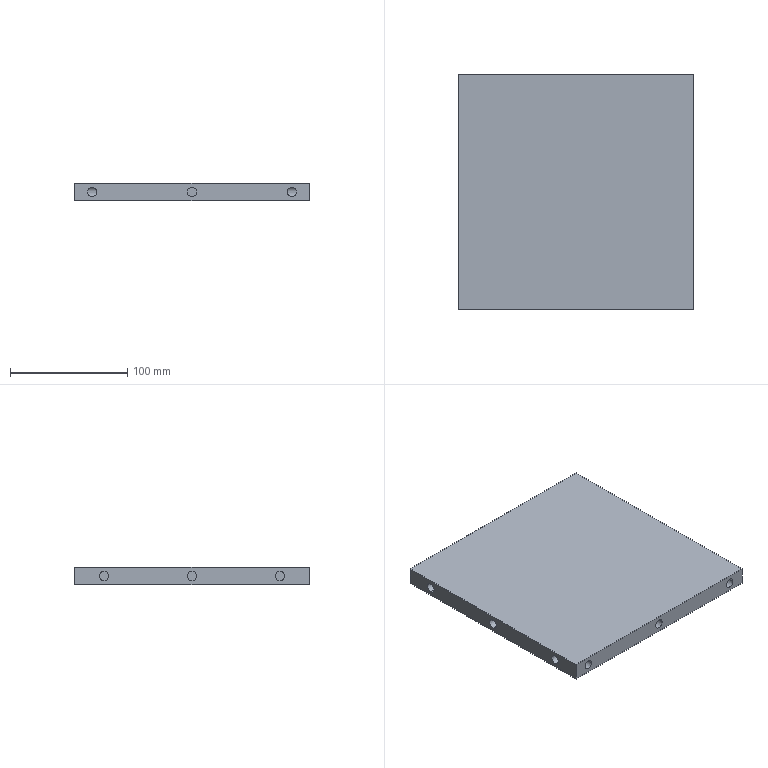Part | SolidWorks | features MirrorPattern 4, LPattern 2, Cut 1, Extrusion 1, ICE 1 | 1 solid | 42 faces | box 200 x 200 x 15 mm | volume 585603 mm3 | cylinder 28 | plane 14 | commonest cylinder face diameters 8 x28
STEP:
#1=CARTESIAN_POINT('',(-85.,-75.,3.5));
#2=VERTEX_POINT('',#1);
#3=CARTESIAN_POINT('',(-89.,-79.,7.5));
#4=VERTEX_POINT('',#3);
#5=CARTESIAN_POINT('',(-85.,-75.,3.5));
#6=CARTESIAN_POINT('',(-87.343,-77.343,3.5));
#7=CARTESIAN_POINT('',(-89.,-79.,5.157));
#8=CARTESIAN_POINT('',(-89.,-79.,7.5));
#9=(BOUNDED_CURVE()B_SPLINE_CURVE(3,(#5,#6,#7,#8),.UNSPECIFIED.,.F.,.F.)B_SPLINE_CURVE_WITH_KNOTS((4,4),(4.712,6.283),.UNSPECIFIED.)CURVE()GEOMETRIC_REPRESENTATION_ITEM()RATIONAL_B_SPLINE_CURVE((1.,0.8047,0.8047,1.))REPRESENTATION_ITEM(''));
#10=EDGE_CURVE('',#2,#4,#9,.T.);
#11=ORIENTED_EDGE('',*,*,#10,.T.);
#12=CARTESIAN_POINT('',(-89.,-100.,7.5));
#13=VERTEX_POINT('',#12);
#14=CARTESIAN_POINT('',(-89.,-75.,7.5));
#15=DIRECTION('',(0.,-1.,0.));
#16=VECTOR('',#15,1000.);
#17=LINE('',#14,#16);
#18=EDGE_CURVE('',#4,#13,#17,.T.);
#19=ORIENTED_EDGE('',*,*,#18,.T.);
#20=CARTESIAN_POINT('',(-81.,-100.,7.5));
#21=VERTEX_POINT('',#20);
#22=CARTESIAN_POINT('',(-85.,-100.,7.5));
#23=DIRECTION('',(0.,-1.,0.));
#24=DIRECTION('',(1.,0.,0.));
#25=AXIS2_PLACEMENT_3D('',#22,#23,#24);
#26=CIRCLE('',#25,4.);
#27=EDGE_CURVE('',#13,#21,#26,.T.);
#28=ORIENTED_EDGE('',*,*,#27,.T.);
#29=CARTESIAN_POINT('',(-81.,-79.,7.5));
#30=VERTEX_POINT('',#29);
#31=CARTESIAN_POINT('',(-81.,-75.,7.5));
#32=DIRECTION('',(0.,-1.,0.));
#33=VECTOR('',#32,1000.);
#34=LINE('',#31,#33);
#35=EDGE_CURVE('',#30,#21,#34,.T.);
#36=ORIENTED_EDGE('',*,*,#35,.F.);
#37=CARTESIAN_POINT('',(-81.,-79.,7.5));
#38=CARTESIAN_POINT('',(-81.,-79.,5.157));
#39=CARTESIAN_POINT('',(-82.657,-77.343,3.5));
#40=CARTESIAN_POINT('',(-85.,-75.,3.5));
#41=(BOUNDED_CURVE()B_SPLINE_CURVE(3,(#37,#38,#39,#40),.UNSPECIFIED.,.F.,.F.)B_SPLINE_CURVE_WITH_KNOTS((4,4),(3.142,4.712),.UNSPECIFIED.)CURVE()GEOMETRIC_REPRESENTATION_ITEM()RATIONAL_B_SPLINE_CURVE((1.,0.8047,0.8047,1.))REPRESENTATION_ITEM(''));
#42=EDGE_CURVE('',#30,#2,#41,.T.);
#43=ORIENTED_EDGE('',*,*,#42,.T.);
#44=EDGE_LOOP('',(#11,#19,#28,#36,#43));
#45=FACE_OUTER_BOUND('',#44,.T.);
#46=CARTESIAN_POINT('',(-85.,-75.,7.5));
#47=DIRECTION('',(0.,-1.,0.));
#48=DIRECTION('',(1.,0.,0.));
#49=AXIS2_PLACEMENT_3D('',#46,#47,#48);
#50=CYLINDRICAL_SURFACE('',#49,4.);
#51=ADVANCED_FACE('',(#45),#50,.F.);
#52=CARTESIAN_POINT('',(85.,-75.,3.5));
#53=VERTEX_POINT('',#52);
#54=CARTESIAN_POINT('',(81.,-79.,7.5));
#55=VERTEX_POINT('',#54);
#56=CARTESIAN_POINT('',(85.,-75.,3.5));
#57=CARTESIAN_POINT('',(82.657,-77.343,3.5));
#58=CARTESIAN_POINT('',(81.,-79.,5.157));
#59=CARTESIAN_POINT('',(81.,-79.,7.5));
#60=(BOUNDED_CURVE()B_SPLINE_CURVE(3,(#56,#57,#58,#59),.UNSPECIFIED.,.F.,.F.)B_SPLINE_CURVE_WITH_KNOTS((4,4),(1.571,3.142),.UNSPECIFIED.)CURVE()GEOMETRIC_REPRESENTATION_ITEM()RATIONAL_B_SPLINE_CURVE((1.,0.8047,0.8047,1.))REPRESENTATION_ITEM(''));
#61=EDGE_CURVE('',#53,#55,#60,.T.);
#62=ORIENTED_EDGE('',*,*,#61,.T.);
#63=CARTESIAN_POINT('',(81.,-100.,7.5));
#64=VERTEX_POINT('',#63);
#65=CARTESIAN_POINT('',(81.,-75.,7.5));
#66=DIRECTION('',(0.,-1.,0.));
#67=VECTOR('',#66,1000.);
#68=LINE('',#65,#67);
#69=EDGE_CURVE('',#55,#64,#68,.T.);
#70=ORIENTED_EDGE('',*,*,#69,.T.);
#71=CARTESIAN_POINT('',(89.,-100.,7.5));
#72=VERTEX_POINT('',#71);
#73=CARTESIAN_POINT('',(85.,-100.,7.5));
#74=DIRECTION('',(0.,1.,0.));
#75=DIRECTION('',(-1.,0.,0.));
#76=AXIS2_PLACEMENT_3D('',#73,#74,#75);
#77=CIRCLE('',#76,4.);
#78=EDGE_CURVE('',#72,#64,#77,.T.);
#79=ORIENTED_EDGE('',*,*,#78,.F.);
#80=CARTESIAN_POINT('',(89.,-79.,7.5));
#81=VERTEX_POINT('',#80);
#82=CARTESIAN_POINT('',(89.,-75.,7.5));
#83=DIRECTION('',(0.,-1.,0.));
#84=VECTOR('',#83,1000.);
#85=LINE('',#82,#84);
#86=EDGE_CURVE('',#81,#72,#85,.T.);
#87=ORIENTED_EDGE('',*,*,#86,.F.);
#88=CARTESIAN_POINT('',(89.,-79.,7.5));
#89=CARTESIAN_POINT('',(89.,-79.,5.157));
#90=CARTESIAN_POINT('',(87.343,-77.343,3.5));
#91=CARTESIAN_POINT('',(85.,-75.,3.5));
#92=(BOUNDED_CURVE()B_SPLINE_CURVE(3,(#88,#89,#90,#91),.UNSPECIFIED.,.F.,.F.)B_SPLINE_CURVE_WITH_KNOTS((4,4),(0.,1.571),.UNSPECIFIED.)CURVE()GEOMETRIC_REPRESENTATION_ITEM()RATIONAL_B_SPLINE_CURVE((1.,0.8047,0.8047,1.))REPRESENTATION_ITEM(''));
#93=EDGE_CURVE('',#81,#53,#92,.T.);
#94=ORIENTED_EDGE('',*,*,#93,.T.);
#95=EDGE_LOOP('',(#62,#70,#79,#87,#94));
#96=FACE_OUTER_BOUND('',#95,.T.);
#97=CARTESIAN_POINT('',(85.,-75.,7.5));
#98=DIRECTION('',(0.,-1.,0.));
#99=DIRECTION('',(1.,0.,0.));
#100=AXIS2_PLACEMENT_3D('',#97,#98,#99);
#101=CYLINDRICAL_SURFACE('',#100,4.);
#102=ADVANCED_FACE('',(#96),#101,.F.);
#103=CARTESIAN_POINT('',(4.,-75.,7.5));
#104=VERTEX_POINT('',#103);
#105=CARTESIAN_POINT('',(-4.,-75.,7.5));
#106=VERTEX_POINT('',#105);
#107=CARTESIAN_POINT('',(0.,-75.,7.5));
#108=DIRECTION('',(0.,1.,0.));
#109=DIRECTION('',(-1.,0.,0.));
#110=AXIS2_PLACEMENT_3D('',#107,#108,#109);
#111=CIRCLE('',#110,4.);
#112=EDGE_CURVE('',#104,#106,#111,.T.);
#113=ORIENTED_EDGE('',*,*,#112,.T.);
#114=CARTESIAN_POINT('',(-4.,-100.,7.5));
#115=VERTEX_POINT('',#114);
#116=CARTESIAN_POINT('',(-4.,-75.,7.5));
#117=DIRECTION('',(0.,-1.,0.));
#118=VECTOR('',#117,1000.);
#119=LINE('',#116,#118);
#120=EDGE_CURVE('',#106,#115,#119,.T.);
#121=ORIENTED_EDGE('',*,*,#120,.T.);
#122=CARTESIAN_POINT('',(4.,-100.,7.5));
#123=VERTEX_POINT('',#122);
#124=CARTESIAN_POINT('',(0.,-100.,7.5));
#125=DIRECTION('',(0.,1.,0.));
#126=DIRECTION('',(-1.,0.,0.));
#127=AXIS2_PLACEMENT_3D('',#124,#125,#126);
#128=CIRCLE('',#127,4.);
#129=EDGE_CURVE('',#123,#115,#128,.T.);
#130=ORIENTED_EDGE('',*,*,#129,.F.);
#131=CARTESIAN_POINT('',(4.,-75.,7.5));
#132=DIRECTION('',(0.,-1.,0.));
#133=VECTOR('',#132,1000.);
#134=LINE('',#131,#133);
#135=EDGE_CURVE('',#104,#123,#134,.T.);
#136=ORIENTED_EDGE('',*,*,#135,.F.);
#137=EDGE_LOOP('',(#113,#121,#130,#136));
#138=FACE_OUTER_BOUND('',#137,.T.);
#139=CARTESIAN_POINT('',(0.,-75.,7.5));
#140=DIRECTION('',(0.,-1.,0.));
#141=DIRECTION('',(1.,0.,0.));
#142=AXIS2_PLACEMENT_3D('',#139,#140,#141);
#143=CYLINDRICAL_SURFACE('',#142,4.);
#144=ADVANCED_FACE('',(#138),#143,.F.);
#145=CARTESIAN_POINT('',(-85.,75.,3.5));
#146=VERTEX_POINT('',#145);
#147=CARTESIAN_POINT('',(-81.,79.,7.5));
#148=VERTEX_POINT('',#147);
#149=CARTESIAN_POINT('',(-85.,75.,3.5));
#150=CARTESIAN_POINT('',(-82.657,77.343,3.5));
#151=CARTESIAN_POINT('',(-81.,79.,5.157));
#152=CARTESIAN_POINT('',(-81.,79.,7.5));
#153=(BOUNDED_CURVE()B_SPLINE_CURVE(3,(#149,#150,#151,#152),.UNSPECIFIED.,.F.,.F.)B_SPLINE_CURVE_WITH_KNOTS((4,4),(1.571,3.142),.UNSPECIFIED.)CURVE()GEOMETRIC_REPRESENTATION_ITEM()RATIONAL_B_SPLINE_CURVE((1.,0.8047,0.8047,1.))REPRESENTATION_ITEM(''));
#154=EDGE_CURVE('',#146,#148,#153,.T.);
#155=ORIENTED_EDGE('',*,*,#154,.T.);
#156=CARTESIAN_POINT('',(-81.,100.,7.5));
#157=VERTEX_POINT('',#156);
#158=CARTESIAN_POINT('',(-81.,75.,7.5));
#159=DIRECTION('',(0.,1.,0.));
#160=VECTOR('',#159,1000.);
#161=LINE('',#158,#160);
#162=EDGE_CURVE('',#148,#157,#161,.T.);
#163=ORIENTED_EDGE('',*,*,#162,.T.);
#164=CARTESIAN_POINT('',(-89.,100.,7.5));
#165=VERTEX_POINT('',#164);
#166=CARTESIAN_POINT('',(-85.,100.,7.5));
#167=DIRECTION('',(0.,-1.,0.));
#168=DIRECTION('',(1.,0.,0.));
#169=AXIS2_PLACEMENT_3D('',#166,#167,#168);
#170=CIRCLE('',#169,4.);
#171=EDGE_CURVE('',#165,#157,#170,.T.);
#172=ORIENTED_EDGE('',*,*,#171,.F.);
#173=CARTESIAN_POINT('',(-89.,79.,7.5));
#174=VERTEX_POINT('',#173);
#175=CARTESIAN_POINT('',(-89.,75.,7.5));
#176=DIRECTION('',(0.,1.,0.));
#177=VECTOR('',#176,1000.);
#178=LINE('',#175,#177);
#179=EDGE_CURVE('',#174,#165,#178,.T.);
#180=ORIENTED_EDGE('',*,*,#179,.F.);
#181=CARTESIAN_POINT('',(-89.,79.,7.5));
#182=CARTESIAN_POINT('',(-89.,79.,5.157));
#183=CARTESIAN_POINT('',(-87.343,77.343,3.5));
#184=CARTESIAN_POINT('',(-85.,75.,3.5));
#185=(BOUNDED_CURVE()B_SPLINE_CURVE(3,(#181,#182,#183,#184),.UNSPECIFIED.,.F.,.F.)B_SPLINE_CURVE_WITH_KNOTS((4,4),(0.,1.571),.UNSPECIFIED.)CURVE()GEOMETRIC_REPRESENTATION_ITEM()RATIONAL_B_SPLINE_CURVE((1.,0.8047,0.8047,1.))REPRESENTATION_ITEM(''));
#186=EDGE_CURVE('',#174,#146,#185,.T.);
#187=ORIENTED_EDGE('',*,*,#186,.T.);
#188=EDGE_LOOP('',(#155,#163,#172,#180,#187));
#189=FACE_OUTER_BOUND('',#188,.T.);
#190=CARTESIAN_POINT('',(-85.,75.,7.5));
#191=DIRECTION('',(0.,1.,0.));
#192=DIRECTION('',(-1.,0.,0.));
#193=AXIS2_PLACEMENT_3D('',#190,#191,#192);
#194=CYLINDRICAL_SURFACE('',#193,4.);
#195=ADVANCED_FACE('',(#189),#194,.F.);
#196=CARTESIAN_POINT('',(85.,75.,3.5));
#197=VERTEX_POINT('',#196);
#198=CARTESIAN_POINT('',(89.,79.,7.5));
#199=VERTEX_POINT('',#198);
#200=CARTESIAN_POINT('',(85.,75.,3.5));
#201=CARTESIAN_POINT('',(87.343,77.343,3.5));
#202=CARTESIAN_POINT('',(89.,79.,5.157));
#203=CARTESIAN_POINT('',(89.,79.,7.5));
#204=(BOUNDED_CURVE()B_SPLINE_CURVE(3,(#200,#201,#202,#203),.UNSPECIFIED.,.F.,.F.)B_SPLINE_CURVE_WITH_KNOTS((4,4),(4.712,6.283),.UNSPECIFIED.)CURVE()GEOMETRIC_REPRESENTATION_ITEM()RATIONAL_B_SPLINE_CURVE((1.,0.8047,0.8047,1.))REPRESENTATION_ITEM(''));
#205=EDGE_CURVE('',#197,#199,#204,.T.);
#206=ORIENTED_EDGE('',*,*,#205,.T.);
#207=CARTESIAN_POINT('',(89.,100.,7.5));
#208=VERTEX_POINT('',#207);
#209=CARTESIAN_POINT('',(89.,75.,7.5));
#210=DIRECTION('',(0.,1.,0.));
#211=VECTOR('',#210,1000.);
#212=LINE('',#209,#211);
#213=EDGE_CURVE('',#199,#208,#212,.T.);
#214=ORIENTED_EDGE('',*,*,#213,.T.);
#215=CARTESIAN_POINT('',(81.,100.,7.5));
#216=VERTEX_POINT('',#215);
#217=CARTESIAN_POINT('',(85.,100.,7.5));
#218=DIRECTION('',(0.,1.,0.));
#219=DIRECTION('',(-1.,0.,0.));
#220=AXIS2_PLACEMENT_3D('',#217,#218,#219);
#221=CIRCLE('',#220,4.);
#222=EDGE_CURVE('',#208,#216,#221,.T.);
#223=ORIENTED_EDGE('',*,*,#222,.T.);
#224=CARTESIAN_POINT('',(81.,79.,7.5));
#225=VERTEX_POINT('',#224);
#226=CARTESIAN_POINT('',(81.,75.,7.5));
#227=DIRECTION('',(0.,1.,0.));
#228=VECTOR('',#227,1000.);
#229=LINE('',#226,#228);
#230=EDGE_CURVE('',#225,#216,#229,.T.);
#231=ORIENTED_EDGE('',*,*,#230,.F.);
#232=CARTESIAN_POINT('',(81.,79.,7.5));
#233=CARTESIAN_POINT('',(81.,79.,5.157));
#234=CARTESIAN_POINT('',(82.657,77.343,3.5));
#235=CARTESIAN_POINT('',(85.,75.,3.5));
#236=(BOUNDED_CURVE()B_SPLINE_CURVE(3,(#232,#233,#234,#235),.UNSPECIFIED.,.F.,.F.)B_SPLINE_CURVE_WITH_KNOTS((4,4),(3.142,4.712),.UNSPECIFIED.)CURVE()GEOMETRIC_REPRESENTATION_ITEM()RATIONAL_B_SPLINE_CURVE((1.,0.8047,0.8047,1.))REPRESENTATION_ITEM(''));
#237=EDGE_CURVE('',#225,#197,#236,.T.);
#238=ORIENTED_EDGE('',*,*,#237,.T.);
#239=EDGE_LOOP('',(#206,#214,#223,#231,#238));
#240=FACE_OUTER_BOUND('',#239,.T.);
#241=CARTESIAN_POINT('',(85.,75.,7.5));
#242=DIRECTION('',(0.,1.,0.));
#243=DIRECTION('',(-1.,0.,0.));
#244=AXIS2_PLACEMENT_3D('',#241,#242,#243);
#245=CYLINDRICAL_SURFACE('',#244,4.);
#246=ADVANCED_FACE('',(#240),#245,.F.);
#247=CARTESIAN_POINT('',(4.,75.,7.5));
#248=VERTEX_POINT('',#247);
#249=CARTESIAN_POINT('',(-4.,75.,7.5));
#250=VERTEX_POINT('',#249);
#251=CARTESIAN_POINT('',(0.,75.,7.5));
#252=DIRECTION('',(0.,1.,0.));
#253=DIRECTION('',(-1.,0.,0.));
#254=AXIS2_PLACEMENT_3D('',#251,#252,#253);
#255=CIRCLE('',#254,4.);
#256=EDGE_CURVE('',#248,#250,#255,.T.);
#257=ORIENTED_EDGE('',*,*,#256,.F.);
#258=CARTESIAN_POINT('',(4.,100.,7.5));
#259=VERTEX_POINT('',#258);
#260=CARTESIAN_POINT('',(4.,75.,7.5));
#261=DIRECTION('',(0.,1.,0.));
#262=VECTOR('',#261,1000.);
#263=LINE('',#260,#262);
#264=EDGE_CURVE('',#248,#259,#263,.T.);
#265=ORIENTED_EDGE('',*,*,#264,.T.);
#266=CARTESIAN_POINT('',(-4.,100.,7.5));
#267=VERTEX_POINT('',#266);
#268=CARTESIAN_POINT('',(0.,100.,7.5));
#269=DIRECTION('',(0.,1.,0.));
#270=DIRECTION('',(-1.,0.,0.));
#271=AXIS2_PLACEMENT_3D('',#268,#269,#270);
#272=CIRCLE('',#271,4.);
#273=EDGE_CURVE('',#259,#267,#272,.T.);
#274=ORIENTED_EDGE('',*,*,#273,.T.);
#275=CARTESIAN_POINT('',(-4.,75.,7.5));
#276=DIRECTION('',(0.,1.,0.));
#277=VECTOR('',#276,1000.);
#278=LINE('',#275,#277);
#279=EDGE_CURVE('',#250,#267,#278,.T.);
#280=ORIENTED_EDGE('',*,*,#279,.F.);
#281=EDGE_LOOP('',(#257,#265,#274,#280));
#282=FACE_OUTER_BOUND('',#281,.T.);
#283=CARTESIAN_POINT('',(0.,75.,7.5));
#284=DIRECTION('',(0.,1.,0.));
#285=DIRECTION('',(-1.,0.,0.));
#286=AXIS2_PLACEMENT_3D('',#283,#284,#285);
#287=CYLINDRICAL_SURFACE('',#286,4.);
#288=ADVANCED_FACE('',(#282),#287,.F.);
#289=CARTESIAN_POINT('',(-75.,-75.,11.5));
#290=VERTEX_POINT('',#289);
#291=CARTESIAN_POINT('',(-75.,-75.,3.5));
#292=VERTEX_POINT('',#291);
#293=CARTESIAN_POINT('',(-75.,-75.,7.5));
#294=DIRECTION('',(1.,0.,0.));
#295=DIRECTION('',(0.,0.,-1.));
#296=AXIS2_PLACEMENT_3D('',#293,#294,#295);
#297=CIRCLE('',#296,4.);
#298=EDGE_CURVE('',#290,#292,#297,.T.);
#299=ORIENTED_EDGE('',*,*,#298,.T.);
#300=CARTESIAN_POINT('',(-75.,-75.,3.5));
#301=DIRECTION('',(-1.,0.,0.));
#302=VECTOR('',#301,1000.);
#303=LINE('',#300,#302);
#304=EDGE_CURVE('',#292,#2,#303,.T.);
#305=ORIENTED_EDGE('',*,*,#304,.T.);
#306=ORIENTED_EDGE('',*,*,#42,.F.);
#307=CARTESIAN_POINT('',(-85.,-75.,11.5));
#308=VERTEX_POINT('',#307);
#309=CARTESIAN_POINT('',(-85.,-75.,11.5));
#310=CARTESIAN_POINT('',(-82.657,-77.343,11.5));
#311=CARTESIAN_POINT('',(-81.,-79.,9.843));
#312=CARTESIAN_POINT('',(-81.,-79.,7.5));
#313=(BOUNDED_CURVE()B_SPLINE_CURVE(3,(#309,#310,#311,#312),.UNSPECIFIED.,.F.,.F.)B_SPLINE_CURVE_WITH_KNOTS((4,4),(1.571,3.142),.UNSPECIFIED.)CURVE()GEOMETRIC_REPRESENTATION_ITEM()RATIONAL_B_SPLINE_CURVE((1.,0.8047,0.8047,1.))REPRESENTATION_ITEM(''));
#314=EDGE_CURVE('',#308,#30,#313,.T.);
#315=ORIENTED_EDGE('',*,*,#314,.F.);
#316=CARTESIAN_POINT('',(-75.,-75.,11.5));
#317=DIRECTION('',(-1.,0.,0.));
#318=VECTOR('',#317,1000.);
#319=LINE('',#316,#318);
#320=EDGE_CURVE('',#290,#308,#319,.T.);
#321=ORIENTED_EDGE('',*,*,#320,.F.);
#322=EDGE_LOOP('',(#299,#305,#306,#315,#321));
#323=FACE_OUTER_BOUND('',#322,.T.);
#324=CARTESIAN_POINT('',(-75.,-75.,7.5));
#325=DIRECTION('',(-1.,0.,0.));
#326=DIRECTION('',(0.,0.,1.));
#327=AXIS2_PLACEMENT_3D('',#324,#325,#326);
#328=CYLINDRICAL_SURFACE('',#327,4.);
#329=ADVANCED_FACE('',(#323),#328,.F.);
#330=ORIENTED_EDGE('',*,*,#10,.F.);
#331=CARTESIAN_POINT('',(-100.,-75.,3.5));
#332=VERTEX_POINT('',#331);
#333=CARTESIAN_POINT('',(-75.,-75.,3.5));
#334=DIRECTION('',(-1.,0.,0.));
#335=VECTOR('',#334,1000.);
#336=LINE('',#333,#335);
#337=EDGE_CURVE('',#2,#332,#336,.T.);
#338=ORIENTED_EDGE('',*,*,#337,.T.);
#339=CARTESIAN_POINT('',(-100.,-75.,11.5));
#340=VERTEX_POINT('',#339);
#341=CARTESIAN_POINT('',(-100.,-75.,7.5));
#342=DIRECTION('',(1.,0.,0.));
#343=DIRECTION('',(0.,0.,-1.));
#344=AXIS2_PLACEMENT_3D('',#341,#342,#343);
#345=CIRCLE('',#344,4.);
#346=EDGE_CURVE('',#340,#332,#345,.T.);
#347=ORIENTED_EDGE('',*,*,#346,.F.);
#348=CARTESIAN_POINT('',(-75.,-75.,11.5));
#349=DIRECTION('',(-1.,0.,0.));
#350=VECTOR('',#349,1000.);
#351=LINE('',#348,#350);
#352=EDGE_CURVE('',#308,#340,#351,.T.);
#353=ORIENTED_EDGE('',*,*,#352,.F.);
#354=CARTESIAN_POINT('',(-89.,-79.,7.5));
#355=CARTESIAN_POINT('',(-89.,-79.,9.843));
#356=CARTESIAN_POINT('',(-87.343,-77.343,11.5));
#357=CARTESIAN_POINT('',(-85.,-75.,11.5));
#358=(BOUNDED_CURVE()B_SPLINE_CURVE(3,(#354,#355,#356,#357),.UNSPECIFIED.,.F.,.F.)B_SPLINE_CURVE_WITH_KNOTS((4,4),(0.,1.571),.UNSPECIFIED.)CURVE()GEOMETRIC_REPRESENTATION_ITEM()RATIONAL_B_SPLINE_CURVE((1.,0.8047,0.8047,1.))REPRESENTATION_ITEM(''));
#359=EDGE_CURVE('',#4,#308,#358,.T.);
#360=ORIENTED_EDGE('',*,*,#359,.F.);
#361=EDGE_LOOP('',(#330,#338,#347,#353,#360));
#362=FACE_OUTER_BOUND('',#361,.T.);
#363=CARTESIAN_POINT('',(-75.,-75.,7.5));
#364=DIRECTION('',(-1.,0.,0.));
#365=DIRECTION('',(0.,0.,1.));
#366=AXIS2_PLACEMENT_3D('',#363,#364,#365);
#367=CYLINDRICAL_SURFACE('',#366,4.);
#368=ADVANCED_FACE('',(#362),#367,.F.);
#369=CARTESIAN_POINT('',(-75.,0.,11.5));
#370=VERTEX_POINT('',#369);
#371=CARTESIAN_POINT('',(-75.,0.,3.5));
#372=VERTEX_POINT('',#371);
#373=CARTESIAN_POINT('',(-75.,0.,7.5));
#374=DIRECTION('',(1.,0.,0.));
#375=DIRECTION('',(0.,0.,-1.));
#376=AXIS2_PLACEMENT_3D('',#373,#374,#375);
#377=CIRCLE('',#376,4.);
#378=EDGE_CURVE('',#370,#372,#377,.T.);
#379=ORIENTED_EDGE('',*,*,#378,.T.);
#380=CARTESIAN_POINT('',(-100.,0.,3.5));
#381=VERTEX_POINT('',#380);
#382=CARTESIAN_POINT('',(-75.,0.,3.5));
#383=DIRECTION('',(-1.,0.,0.));
#384=VECTOR('',#383,1000.);
#385=LINE('',#382,#384);
#386=EDGE_CURVE('',#372,#381,#385,.T.);
#387=ORIENTED_EDGE('',*,*,#386,.T.);
#388=CARTESIAN_POINT('',(-100.,0.,11.5));
#389=VERTEX_POINT('',#388);
#390=CARTESIAN_POINT('',(-100.,0.,7.5));
#391=DIRECTION('',(1.,0.,0.));
#392=DIRECTION('',(0.,0.,-1.));
#393=AXIS2_PLACEMENT_3D('',#390,#391,#392);
#394=CIRCLE('',#393,4.);
#395=EDGE_CURVE('',#389,#381,#394,.T.);
#396=ORIENTED_EDGE('',*,*,#395,.F.);
#397=CARTESIAN_POINT('',(-75.,0.,11.5));
#398=DIRECTION('',(-1.,0.,0.));
#399=VECTOR('',#398,1000.);
#400=LINE('',#397,#399);
#401=EDGE_CURVE('',#370,#389,#400,.T.);
#402=ORIENTED_EDGE('',*,*,#401,.F.);
#403=EDGE_LOOP('',(#379,#387,#396,#402));
#404=FACE_OUTER_BOUND('',#403,.T.);
#405=CARTESIAN_POINT('',(-75.,0.,7.5));
#406=DIRECTION('',(-1.,0.,0.));
#407=DIRECTION('',(0.,0.,1.));
#408=AXIS2_PLACEMENT_3D('',#405,#406,#407);
#409=CYLINDRICAL_SURFACE('',#408,4.);
#410=ADVANCED_FACE('',(#404),#409,.F.);
#411=CARTESIAN_POINT('',(75.,75.,3.5));
#412=VERTEX_POINT('',#411);
#413=CARTESIAN_POINT('',(75.,75.,11.5));
#414=VERTEX_POINT('',#413);
#415=CARTESIAN_POINT('',(75.,75.,7.5));
#416=DIRECTION('',(-1.,0.,0.));
#417=DIRECTION('',(0.,0.,-1.));
#418=AXIS2_PLACEMENT_3D('',#415,#416,#417);
#419=CIRCLE('',#418,4.);
#420=EDGE_CURVE('',#412,#414,#419,.T.);
#421=ORIENTED_EDGE('',*,*,#420,.T.);
#422=CARTESIAN_POINT('',(85.,75.,11.5));
#423=VERTEX_POINT('',#422);
#424=CARTESIAN_POINT('',(75.,75.,11.5));
#425=DIRECTION('',(1.,0.,0.));
#426=VECTOR('',#425,1000.);
#427=LINE('',#424,#426);
#428=EDGE_CURVE('',#414,#423,#427,.T.);
#429=ORIENTED_EDGE('',*,*,#428,.T.);
#430=CARTESIAN_POINT('',(100.,75.,11.5));
#431=VERTEX_POINT('',#430);
#432=CARTESIAN_POINT('',(75.,75.,11.5));
#433=DIRECTION('',(1.,0.,0.));
#434=VECTOR('',#433,1000.);
#435=LINE('',#432,#434);
#436=EDGE_CURVE('',#423,#431,#435,.T.);
#437=ORIENTED_EDGE('',*,*,#436,.T.);
#438=CARTESIAN_POINT('',(100.,75.,3.5));
#439=VERTEX_POINT('',#438);
#440=CARTESIAN_POINT('',(100.,75.,7.5));
#441=DIRECTION('',(-1.,0.,0.));
#442=DIRECTION('',(0.,0.,-1.));
#443=AXIS2_PLACEMENT_3D('',#440,#441,#442);
#444=CIRCLE('',#443,4.);
#445=EDGE_CURVE('',#439,#431,#444,.T.);
#446=ORIENTED_EDGE('',*,*,#445,.F.);
#447=CARTESIAN_POINT('',(75.,75.,3.5));
#448=DIRECTION('',(1.,0.,0.));
#449=VECTOR('',#448,1000.);
#450=LINE('',#447,#449);
#451=EDGE_CURVE('',#197,#439,#450,.T.);
#452=ORIENTED_EDGE('',*,*,#451,.F.);
#453=CARTESIAN_POINT('',(75.,75.,3.5));
#454=DIRECTION('',(1.,0.,0.));
#455=VECTOR('',#454,1000.);
#456=LINE('',#453,#455);
#457=EDGE_CURVE('',#412,#197,#456,.T.);
#458=ORIENTED_EDGE('',*,*,#457,.F.);
#459=EDGE_LOOP('',(#421,#429,#437,#446,#452,#458));
#460=FACE_OUTER_BOUND('',#459,.T.);
#461=CARTESIAN_POINT('',(75.,75.,7.5));
#462=DIRECTION('',(1.,0.,0.));
#463=DIRECTION('',(0.,0.,-1.));
#464=AXIS2_PLACEMENT_3D('',#461,#462,#463);
#465=CYLINDRICAL_SURFACE('',#464,4.);
#466=ADVANCED_FACE('',(#460),#465,.F.);
#467=ORIENTED_EDGE('',*,*,#428,.F.);
#468=CARTESIAN_POINT('',(75.,75.,7.5));
#469=DIRECTION('',(-1.,0.,0.));
#470=DIRECTION('',(0.,0.,-1.));
#471=AXIS2_PLACEMENT_3D('',#468,#469,#470);
#472=CIRCLE('',#471,4.);
#473=EDGE_CURVE('',#414,#412,#472,.T.);
#474=ORIENTED_EDGE('',*,*,#473,.T.);
#475=ORIENTED_EDGE('',*,*,#457,.T.);
#476=ORIENTED_EDGE('',*,*,#237,.F.);
#477=CARTESIAN_POINT('',(85.,75.,11.5));
#478=CARTESIAN_POINT('',(82.657,77.343,11.5));
#479=CARTESIAN_POINT('',(81.,79.,9.843));
#480=CARTESIAN_POINT('',(81.,79.,7.5));
#481=(BOUNDED_CURVE()B_SPLINE_CURVE(3,(#477,#478,#479,#480),.UNSPECIFIED.,.F.,.T.)B_SPLINE_CURVE_WITH_KNOTS((4,4),(1.571,3.142),.UNSPECIFIED.)CURVE()GEOMETRIC_REPRESENTATION_ITEM()RATIONAL_B_SPLINE_CURVE((1.,0.8047,0.8047,1.))REPRESENTATION_ITEM(''));
#482=EDGE_CURVE('',#423,#225,#481,.T.);
#483=ORIENTED_EDGE('',*,*,#482,.F.);
#484=EDGE_LOOP('',(#467,#474,#475,#476,#483));
#485=FACE_OUTER_BOUND('',#484,.T.);
#486=CARTESIAN_POINT('',(75.,75.,7.5));
#487=DIRECTION('',(1.,0.,0.));
#488=DIRECTION('',(0.,0.,-1.));
#489=AXIS2_PLACEMENT_3D('',#486,#487,#488);
#490=CYLINDRICAL_SURFACE('',#489,4.);
#491=ADVANCED_FACE('',(#485),#490,.F.);
#492=CARTESIAN_POINT('',(75.,0.,11.5));
#493=VERTEX_POINT('',#492);
#494=CARTESIAN_POINT('',(75.,0.,3.5));
#495=VERTEX_POINT('',#494);
#496=CARTESIAN_POINT('',(75.,0.,7.5));
#497=DIRECTION('',(1.,0.,0.));
#498=DIRECTION('',(0.,0.,-1.));
#499=AXIS2_PLACEMENT_3D('',#496,#497,#498);
#500=CIRCLE('',#499,4.);
#501=EDGE_CURVE('',#493,#495,#500,.T.);
#502=ORIENTED_EDGE('',*,*,#501,.F.);
#503=CARTESIAN_POINT('',(100.,0.,11.5));
#504=VERTEX_POINT('',#503);
#505=CARTESIAN_POINT('',(75.,0.,11.5));
#506=DIRECTION('',(1.,0.,0.));
#507=VECTOR('',#506,1000.);
#508=LINE('',#505,#507);
#509=EDGE_CURVE('',#493,#504,#508,.T.);
#510=ORIENTED_EDGE('',*,*,#509,.T.);
#511=CARTESIAN_POINT('',(100.,0.,3.5));
#512=VERTEX_POINT('',#511);
#513=CARTESIAN_POINT('',(100.,0.,7.5));
#514=DIRECTION('',(1.,0.,0.));
#515=DIRECTION('',(0.,0.,-1.));
#516=AXIS2_PLACEMENT_3D('',#513,#514,#515);
#517=CIRCLE('',#516,4.);
#518=EDGE_CURVE('',#504,#512,#517,.T.);
#519=ORIENTED_EDGE('',*,*,#518,.T.);
#520=CARTESIAN_POINT('',(75.,0.,3.5));
#521=DIRECTION('',(1.,0.,0.));
#522=VECTOR('',#521,1000.);
#523=LINE('',#520,#522);
#524=EDGE_CURVE('',#495,#512,#523,.T.);
#525=ORIENTED_EDGE('',*,*,#524,.F.);
#526=EDGE_LOOP('',(#502,#510,#519,#525));
#527=FACE_OUTER_BOUND('',#526,.T.);
#528=CARTESIAN_POINT('',(75.,0.,7.5));
#529=DIRECTION('',(1.,0.,0.));
#530=DIRECTION('',(0.,0.,-1.));
#531=AXIS2_PLACEMENT_3D('',#528,#529,#530);
#532=CYLINDRICAL_SURFACE('',#531,4.);
#533=ADVANCED_FACE('',(#527),#532,.F.);
#534=CARTESIAN_POINT('',(-75.,75.,3.5));
#535=VERTEX_POINT('',#534);
#536=CARTESIAN_POINT('',(-75.,75.,11.5));
#537=VERTEX_POINT('',#536);
#538=CARTESIAN_POINT('',(-75.,75.,7.5));
#539=DIRECTION('',(-1.,0.,0.));
#540=DIRECTION('',(0.,0.,-1.));
#541=AXIS2_PLACEMENT_3D('',#538,#539,#540);
#542=CIRCLE('',#541,4.);
#543=EDGE_CURVE('',#535,#537,#542,.T.);
#544=ORIENTED_EDGE('',*,*,#543,.F.);
#545=CARTESIAN_POINT('',(-75.,75.,3.5));
#546=DIRECTION('',(-1.,0.,0.));
#547=VECTOR('',#546,1000.);
#548=LINE('',#545,#547);
#549=EDGE_CURVE('',#535,#146,#548,.T.);
#550=ORIENTED_EDGE('',*,*,#549,.T.);
#551=CARTESIAN_POINT('',(-100.,75.,3.5));
#552=VERTEX_POINT('',#551);
#553=CARTESIAN_POINT('',(-75.,75.,3.5));
#554=DIRECTION('',(-1.,0.,0.));
#555=VECTOR('',#554,1000.);
#556=LINE('',#553,#555);
#557=EDGE_CURVE('',#146,#552,#556,.T.);
#558=ORIENTED_EDGE('',*,*,#557,.T.);
#559=CARTESIAN_POINT('',(-100.,75.,11.5));
#560=VERTEX_POINT('',#559);
#561=CARTESIAN_POINT('',(-100.,75.,7.5));
#562=DIRECTION('',(-1.,0.,0.));
#563=DIRECTION('',(0.,0.,-1.));
#564=AXIS2_PLACEMENT_3D('',#561,#562,#563);
#565=CIRCLE('',#564,4.);
#566=EDGE_CURVE('',#552,#560,#565,.T.);
#567=ORIENTED_EDGE('',*,*,#566,.T.);
#568=CARTESIAN_POINT('',(-85.,75.,11.5));
#569=VERTEX_POINT('',#568);
#570=CARTESIAN_POINT('',(-75.,75.,11.5));
#571=DIRECTION('',(-1.,0.,0.));
#572=VECTOR('',#571,1000.);
#573=LINE('',#570,#572);
#574=EDGE_CURVE('',#569,#560,#573,.T.);
#575=ORIENTED_EDGE('',*,*,#574,.F.);
#576=CARTESIAN_POINT('',(-75.,75.,11.5));
#577=DIRECTION('',(-1.,0.,0.));
#578=VECTOR('',#577,1000.);
#579=LINE('',#576,#578);
#580=EDGE_CURVE('',#537,#569,#579,.T.);
#581=ORIENTED_EDGE('',*,*,#580,.F.);
#582=EDGE_LOOP('',(#544,#550,#558,#567,#575,#581));
#583=FACE_OUTER_BOUND('',#582,.T.);
#584=CARTESIAN_POINT('',(-75.,75.,7.5));
#585=DIRECTION('',(-1.,0.,0.));
#586=DIRECTION('',(0.,0.,1.));
#587=AXIS2_PLACEMENT_3D('',#584,#585,#586);
#588=CYLINDRICAL_SURFACE('',#587,4.);
#589=ADVANCED_FACE('',(#583),#588,.F.);
#590=ORIENTED_EDGE('',*,*,#549,.F.);
#591=CARTESIAN_POINT('',(-75.,75.,7.5));
#592=DIRECTION('',(-1.,0.,0.));
#593=DIRECTION('',(0.,0.,-1.));
#594=AXIS2_PLACEMENT_3D('',#591,#592,#593);
#595=CIRCLE('',#594,4.);
#596=EDGE_CURVE('',#537,#535,#595,.T.);
#597=ORIENTED_EDGE('',*,*,#596,.F.);
#598=ORIENTED_EDGE('',*,*,#580,.T.);
#599=CARTESIAN_POINT('',(-81.,79.,7.5));
#600=CARTESIAN_POINT('',(-81.,79.,9.843));
#601=CARTESIAN_POINT('',(-82.657,77.343,11.5));
#602=CARTESIAN_POINT('',(-85.,75.,11.5));
#603=(BOUNDED_CURVE()B_SPLINE_CURVE(3,(#599,#600,#601,#602),.UNSPECIFIED.,.F.,.T.)B_SPLINE_CURVE_WITH_KNOTS((4,4),(3.142,4.712),.UNSPECIFIED.)CURVE()GEOMETRIC_REPRESENTATION_ITEM()RATIONAL_B_SPLINE_CURVE((1.,0.8047,0.8047,1.))REPRESENTATION_ITEM(''));
#604=EDGE_CURVE('',#148,#569,#603,.T.);
#605=ORIENTED_EDGE('',*,*,#604,.F.);
#606=ORIENTED_EDGE('',*,*,#154,.F.);
#607=EDGE_LOOP('',(#590,#597,#598,#605,#606));
#608=FACE_OUTER_BOUND('',#607,.T.);
#609=CARTESIAN_POINT('',(-75.,75.,7.5));
#610=DIRECTION('',(-1.,0.,0.));
#611=DIRECTION('',(0.,0.,1.));
#612=AXIS2_PLACEMENT_3D('',#609,#610,#611);
#613=CYLINDRICAL_SURFACE('',#612,4.);
#614=ADVANCED_FACE('',(#608),#613,.F.);
#615=CARTESIAN_POINT('',(75.,-75.,11.5));
#616=VERTEX_POINT('',#615);
#617=CARTESIAN_POINT('',(75.,-75.,3.5));
#618=VERTEX_POINT('',#617);
#619=CARTESIAN_POINT('',(75.,-75.,7.5));
#620=DIRECTION('',(1.,0.,0.));
#621=DIRECTION('',(0.,0.,-1.));
#622=AXIS2_PLACEMENT_3D('',#619,#620,#621);
#623=CIRCLE('',#622,4.);
#624=EDGE_CURVE('',#616,#618,#623,.T.);
#625=ORIENTED_EDGE('',*,*,#624,.F.);
#626=CARTESIAN_POINT('',(85.,-75.,11.5));
#627=VERTEX_POINT('',#626);
#628=CARTESIAN_POINT('',(75.,-75.,11.5));
#629=DIRECTION('',(1.,0.,0.));
#630=VECTOR('',#629,1000.);
#631=LINE('',#628,#630);
#632=EDGE_CURVE('',#616,#627,#631,.T.);
#633=ORIENTED_EDGE('',*,*,#632,.T.);
#634=CARTESIAN_POINT('',(81.,-79.,7.5));
#635=CARTESIAN_POINT('',(81.,-79.,9.843));
#636=CARTESIAN_POINT('',(82.657,-77.343,11.5));
#637=CARTESIAN_POINT('',(85.,-75.,11.5));
#638=(BOUNDED_CURVE()B_SPLINE_CURVE(3,(#634,#635,#636,#637),.UNSPECIFIED.,.F.,.F.)B_SPLINE_CURVE_WITH_KNOTS((4,4),(3.142,4.712),.UNSPECIFIED.)CURVE()GEOMETRIC_REPRESENTATION_ITEM()RATIONAL_B_SPLINE_CURVE((1.,0.8047,0.8047,1.))REPRESENTATION_ITEM(''));
#639=EDGE_CURVE('',#55,#627,#638,.T.);
#640=ORIENTED_EDGE('',*,*,#639,.F.);
#641=ORIENTED_EDGE('',*,*,#61,.F.);
#642=CARTESIAN_POINT('',(75.,-75.,3.5));
#643=DIRECTION('',(1.,0.,0.));
#644=VECTOR('',#643,1000.);
#645=LINE('',#642,#644);
#646=EDGE_CURVE('',#618,#53,#645,.T.);
#647=ORIENTED_EDGE('',*,*,#646,.F.);
#648=EDGE_LOOP('',(#625,#633,#640,#641,#647));
#649=FACE_OUTER_BOUND('',#648,.T.);
#650=CARTESIAN_POINT('',(75.,-75.,7.5));
#651=DIRECTION('',(1.,0.,0.));
#652=DIRECTION('',(0.,0.,-1.));
#653=AXIS2_PLACEMENT_3D('',#650,#651,#652);
#654=CYLINDRICAL_SURFACE('',#653,4.);
#655=ADVANCED_FACE('',(#649),#654,.F.);
#656=CARTESIAN_POINT('',(85.,-75.,11.5));
#657=CARTESIAN_POINT('',(87.343,-77.343,11.5));
#658=CARTESIAN_POINT('',(89.,-79.,9.843));
#659=CARTESIAN_POINT('',(89.,-79.,7.5));
#660=(BOUNDED_CURVE()B_SPLINE_CURVE(3,(#656,#657,#658,#659),.UNSPECIFIED.,.F.,.F.)B_SPLINE_CURVE_WITH_KNOTS((4,4),(4.712,6.283),.UNSPECIFIED.)CURVE()GEOMETRIC_REPRESENTATION_ITEM()RATIONAL_B_SPLINE_CURVE((1.,0.8047,0.8047,1.))REPRESENTATION_ITEM(''));
#661=EDGE_CURVE('',#627,#81,#660,.T.);
#662=ORIENTED_EDGE('',*,*,#661,.F.);
#663=CARTESIAN_POINT('',(100.,-75.,11.5));
#664=VERTEX_POINT('',#663);
#665=CARTESIAN_POINT('',(75.,-75.,11.5));
#666=DIRECTION('',(1.,0.,0.));
#667=VECTOR('',#666,1000.);
#668=LINE('',#665,#667);
#669=EDGE_CURVE('',#627,#664,#668,.T.);
#670=ORIENTED_EDGE('',*,*,#669,.T.);
#671=CARTESIAN_POINT('',(100.,-75.,3.5));
#672=VERTEX_POINT('',#671);
#673=CARTESIAN_POINT('',(100.,-75.,7.5));
#674=DIRECTION('',(1.,0.,0.));
#675=DIRECTION('',(0.,0.,-1.));
#676=AXIS2_PLACEMENT_3D('',#673,#674,#675);
#677=CIRCLE('',#676,4.);
#678=EDGE_CURVE('',#664,#672,#677,.T.);
#679=ORIENTED_EDGE('',*,*,#678,.T.);
#680=CARTESIAN_POINT('',(75.,-75.,3.5));
#681=DIRECTION('',(1.,0.,0.));
#682=VECTOR('',#681,1000.);
#683=LINE('',#680,#682);
#684=EDGE_CURVE('',#53,#672,#683,.T.);
#685=ORIENTED_EDGE('',*,*,#684,.F.);
#686=ORIENTED_EDGE('',*,*,#93,.F.);
#687=EDGE_LOOP('',(#662,#670,#679,#685,#686));
#688=FACE_OUTER_BOUND('',#687,.T.);
#689=CARTESIAN_POINT('',(75.,-75.,7.5));
#690=DIRECTION('',(1.,0.,0.));
#691=DIRECTION('',(0.,0.,-1.));
#692=AXIS2_PLACEMENT_3D('',#689,#690,#691);
#693=CYLINDRICAL_SURFACE('',#692,4.);
#694=ADVANCED_FACE('',(#688),#693,.F.);
#695=CARTESIAN_POINT('',(-85.,-100.,7.5));
#696=DIRECTION('',(0.,-1.,0.));
#697=DIRECTION('',(1.,0.,0.));
#698=AXIS2_PLACEMENT_3D('',#695,#696,#697);
#699=CIRCLE('',#698,4.);
#700=EDGE_CURVE('',#21,#13,#699,.T.);
#701=ORIENTED_EDGE('',*,*,#700,.F.);
#702=ORIENTED_EDGE('',*,*,#27,.F.);
#703=EDGE_LOOP('',(#701,#702));
#704=FACE_BOUND('',#703,.T.);
#705=ORIENTED_EDGE('',*,*,#129,.T.);
#706=CARTESIAN_POINT('',(0.,-100.,7.5));
#707=DIRECTION('',(0.,1.,0.));
#708=DIRECTION('',(-1.,0.,0.));
#709=AXIS2_PLACEMENT_3D('',#706,#707,#708);
#710=CIRCLE('',#709,4.);
#711=EDGE_CURVE('',#115,#123,#710,.T.);
#712=ORIENTED_EDGE('',*,*,#711,.T.);
#713=EDGE_LOOP('',(#705,#712));
#714=FACE_BOUND('',#713,.T.);
#715=CARTESIAN_POINT('',(-100.,-100.,0.));
#716=VERTEX_POINT('',#715);
#717=CARTESIAN_POINT('',(100.,-100.,0.));
#718=VERTEX_POINT('',#717);
#719=CARTESIAN_POINT('',(100.,-100.,0.));
#720=DIRECTION('',(1.,0.,0.));
#721=VECTOR('',#720,1000.);
#722=LINE('',#719,#721);
#723=EDGE_CURVE('',#716,#718,#722,.T.);
#724=ORIENTED_EDGE('',*,*,#723,.T.);
#725=CARTESIAN_POINT('',(100.,-100.,15.));
#726=VERTEX_POINT('',#725);
#727=CARTESIAN_POINT('',(100.,-100.,15.));
#728=DIRECTION('',(0.,0.,-1.));
#729=VECTOR('',#728,1000.);
#730=LINE('',#727,#729);
#731=EDGE_CURVE('',#726,#718,#730,.T.);
#732=ORIENTED_EDGE('',*,*,#731,.F.);
#733=CARTESIAN_POINT('',(-100.,-100.,15.));
#734=VERTEX_POINT('',#733);
#735=CARTESIAN_POINT('',(100.,-100.,15.));
#736=DIRECTION('',(1.,0.,0.));
#737=VECTOR('',#736,1000.);
#738=LINE('',#735,#737);
#739=EDGE_CURVE('',#734,#726,#738,.T.);
#740=ORIENTED_EDGE('',*,*,#739,.F.);
#741=CARTESIAN_POINT('',(-100.,-100.,15.));
#742=DIRECTION('',(0.,0.,-1.));
#743=VECTOR('',#742,1000.);
#744=LINE('',#741,#743);
#745=EDGE_CURVE('',#734,#716,#744,.T.);
#746=ORIENTED_EDGE('',*,*,#745,.T.);
#747=EDGE_LOOP('',(#724,#732,#740,#746));
#748=FACE_OUTER_BOUND('',#747,.T.);
#749=ORIENTED_EDGE('',*,*,#78,.T.);
#750=CARTESIAN_POINT('',(85.,-100.,7.5));
#751=DIRECTION('',(0.,1.,0.));
#752=DIRECTION('',(-1.,0.,0.));
#753=AXIS2_PLACEMENT_3D('',#750,#751,#752);
#754=CIRCLE('',#753,4.);
#755=EDGE_CURVE('',#64,#72,#754,.T.);
#756=ORIENTED_EDGE('',*,*,#755,.T.);
#757=EDGE_LOOP('',(#749,#756));
#758=FACE_BOUND('',#757,.T.);
#759=CARTESIAN_POINT('',(100.,-100.,15.));
#760=DIRECTION('',(0.,1.,0.));
#761=DIRECTION('',(-1.,0.,0.));
#762=AXIS2_PLACEMENT_3D('',#759,#760,#761);
#763=PLANE('',#762);
#764=ADVANCED_FACE('',(#704,#714,#748,#758),#763,.F.);
#765=ORIENTED_EDGE('',*,*,#632,.F.);
#766=CARTESIAN_POINT('',(75.,-75.,7.5));
#767=DIRECTION('',(1.,0.,0.));
#768=DIRECTION('',(0.,0.,-1.));
#769=AXIS2_PLACEMENT_3D('',#766,#767,#768);
#770=CIRCLE('',#769,4.);
#771=EDGE_CURVE('',#618,#616,#770,.T.);
#772=ORIENTED_EDGE('',*,*,#771,.F.);
#773=ORIENTED_EDGE('',*,*,#646,.T.);
#774=ORIENTED_EDGE('',*,*,#684,.T.);
#775=CARTESIAN_POINT('',(100.,-75.,7.5));
#776=DIRECTION('',(1.,0.,0.));
#777=DIRECTION('',(0.,0.,-1.));
#778=AXIS2_PLACEMENT_3D('',#775,#776,#777);
#779=CIRCLE('',#778,4.);
#780=EDGE_CURVE('',#672,#664,#779,.T.);
#781=ORIENTED_EDGE('',*,*,#780,.T.);
#782=ORIENTED_EDGE('',*,*,#669,.F.);
#783=EDGE_LOOP('',(#765,#772,#773,#774,#781,#782));
#784=FACE_OUTER_BOUND('',#783,.T.);
#785=CARTESIAN_POINT('',(75.,-75.,7.5));
#786=DIRECTION('',(1.,0.,0.));
#787=DIRECTION('',(0.,0.,-1.));
#788=AXIS2_PLACEMENT_3D('',#785,#786,#787);
#789=CYLINDRICAL_SURFACE('',#788,4.);
#790=ADVANCED_FACE('',(#784),#789,.F.);
#791=CARTESIAN_POINT('',(100.,100.,0.));
#792=VERTEX_POINT('',#791);
#793=CARTESIAN_POINT('',(-100.,100.,0.));
#794=VERTEX_POINT('',#793);
#795=CARTESIAN_POINT('',(100.,100.,0.));
#796=DIRECTION('',(-1.,0.,0.));
#797=VECTOR('',#796,1000.);
#798=LINE('',#795,#797);
#799=EDGE_CURVE('',#792,#794,#798,.T.);
#800=ORIENTED_EDGE('',*,*,#799,.T.);
#801=CARTESIAN_POINT('',(-100.,100.,15.));
#802=VERTEX_POINT('',#801);
#803=CARTESIAN_POINT('',(-100.,100.,15.));
#804=DIRECTION('',(0.,0.,-1.));
#805=VECTOR('',#804,1000.);
#806=LINE('',#803,#805);
#807=EDGE_CURVE('',#802,#794,#806,.T.);
#808=ORIENTED_EDGE('',*,*,#807,.F.);
#809=CARTESIAN_POINT('',(100.,100.,15.));
#810=VERTEX_POINT('',#809);
#811=CARTESIAN_POINT('',(100.,100.,15.));
#812=DIRECTION('',(-1.,0.,0.));
#813=VECTOR('',#812,1000.);
#814=LINE('',#811,#813);
#815=EDGE_CURVE('',#810,#802,#814,.T.);
#816=ORIENTED_EDGE('',*,*,#815,.F.);
#817=CARTESIAN_POINT('',(100.,100.,15.));
#818=DIRECTION('',(0.,0.,-1.));
#819=VECTOR('',#818,1000.);
#820=LINE('',#817,#819);
#821=EDGE_CURVE('',#810,#792,#820,.T.);
#822=ORIENTED_EDGE('',*,*,#821,.T.);
#823=EDGE_LOOP('',(#800,#808,#816,#822));
#824=FACE_OUTER_BOUND('',#823,.T.);
#825=CARTESIAN_POINT('',(0.,100.,7.5));
#826=DIRECTION('',(0.,1.,0.));
#827=DIRECTION('',(-1.,0.,0.));
#828=AXIS2_PLACEMENT_3D('',#825,#826,#827);
#829=CIRCLE('',#828,4.);
#830=EDGE_CURVE('',#267,#259,#829,.T.);
#831=ORIENTED_EDGE('',*,*,#830,.F.);
#832=ORIENTED_EDGE('',*,*,#273,.F.);
#833=EDGE_LOOP('',(#831,#832));
#834=FACE_BOUND('',#833,.T.);
#835=CARTESIAN_POINT('',(85.,100.,7.5));
#836=DIRECTION('',(0.,1.,0.));
#837=DIRECTION('',(-1.,0.,0.));
#838=AXIS2_PLACEMENT_3D('',#835,#836,#837);
#839=CIRCLE('',#838,4.);
#840=EDGE_CURVE('',#216,#208,#839,.T.);
#841=ORIENTED_EDGE('',*,*,#840,.F.);
#842=ORIENTED_EDGE('',*,*,#222,.F.);
#843=EDGE_LOOP('',(#841,#842));
#844=FACE_BOUND('',#843,.T.);
#845=ORIENTED_EDGE('',*,*,#171,.T.);
#846=CARTESIAN_POINT('',(-85.,100.,7.5));
#847=DIRECTION('',(0.,-1.,0.));
#848=DIRECTION('',(1.,0.,0.));
#849=AXIS2_PLACEMENT_3D('',#846,#847,#848);
#850=CIRCLE('',#849,4.);
#851=EDGE_CURVE('',#157,#165,#850,.T.);
#852=ORIENTED_EDGE('',*,*,#851,.T.);
#853=EDGE_LOOP('',(#845,#852));
#854=FACE_BOUND('',#853,.T.);
#855=CARTESIAN_POINT('',(100.,100.,15.));
#856=DIRECTION('',(0.,-1.,0.));
#857=DIRECTION('',(1.,0.,0.));
#858=AXIS2_PLACEMENT_3D('',#855,#856,#857);
#859=PLANE('',#858);
#860=ADVANCED_FACE('',(#824,#834,#844,#854),#859,.F.);
#861=ORIENTED_EDGE('',*,*,#557,.F.);
#862=ORIENTED_EDGE('',*,*,#186,.F.);
#863=CARTESIAN_POINT('',(-85.,75.,11.5));
#864=CARTESIAN_POINT('',(-87.343,77.343,11.5));
#865=CARTESIAN_POINT('',(-89.,79.,9.843));
#866=CARTESIAN_POINT('',(-89.,79.,7.5));
#867=(BOUNDED_CURVE()B_SPLINE_CURVE(3,(#863,#864,#865,#866),.UNSPECIFIED.,.F.,.T.)B_SPLINE_CURVE_WITH_KNOTS((4,4),(4.712,6.283),.UNSPECIFIED.)CURVE()GEOMETRIC_REPRESENTATION_ITEM()RATIONAL_B_SPLINE_CURVE((1.,0.8047,0.8047,1.))REPRESENTATION_ITEM(''));
#868=EDGE_CURVE('',#569,#174,#867,.T.);
#869=ORIENTED_EDGE('',*,*,#868,.F.);
#870=ORIENTED_EDGE('',*,*,#574,.T.);
#871=CARTESIAN_POINT('',(-100.,75.,7.5));
#872=DIRECTION('',(-1.,0.,0.));
#873=DIRECTION('',(0.,0.,-1.));
#874=AXIS2_PLACEMENT_3D('',#871,#872,#873);
#875=CIRCLE('',#874,4.);
#876=EDGE_CURVE('',#560,#552,#875,.T.);
#877=ORIENTED_EDGE('',*,*,#876,.T.);
#878=EDGE_LOOP('',(#861,#862,#869,#870,#877));
#879=FACE_OUTER_BOUND('',#878,.T.);
#880=CARTESIAN_POINT('',(-75.,75.,7.5));
#881=DIRECTION('',(-1.,0.,0.));
#882=DIRECTION('',(0.,0.,1.));
#883=AXIS2_PLACEMENT_3D('',#880,#881,#882);
#884=CYLINDRICAL_SURFACE('',#883,4.);
#885=ADVANCED_FACE('',(#879),#884,.F.);
#886=ORIENTED_EDGE('',*,*,#876,.F.);
#887=ORIENTED_EDGE('',*,*,#566,.F.);
#888=EDGE_LOOP('',(#886,#887));
#889=FACE_BOUND('',#888,.T.);
#890=ORIENTED_EDGE('',*,*,#395,.T.);
#891=CARTESIAN_POINT('',(-100.,0.,7.5));
#892=DIRECTION('',(1.,0.,0.));
#893=DIRECTION('',(0.,0.,-1.));
#894=AXIS2_PLACEMENT_3D('',#891,#892,#893);
#895=CIRCLE('',#894,4.);
#896=EDGE_CURVE('',#381,#389,#895,.T.);
#897=ORIENTED_EDGE('',*,*,#896,.T.);
#898=EDGE_LOOP('',(#890,#897));
#899=FACE_BOUND('',#898,.T.);
#900=CARTESIAN_POINT('',(-100.,-100.,0.));
#901=DIRECTION('',(0.,-1.,0.));
#902=VECTOR('',#901,1000.);
#903=LINE('',#900,#902);
#904=EDGE_CURVE('',#794,#716,#903,.T.);
#905=ORIENTED_EDGE('',*,*,#904,.T.);
#906=ORIENTED_EDGE('',*,*,#745,.F.);
#907=CARTESIAN_POINT('',(-100.,-100.,15.));
#908=DIRECTION('',(0.,-1.,0.));
#909=VECTOR('',#908,1000.);
#910=LINE('',#907,#909);
#911=EDGE_CURVE('',#802,#734,#910,.T.);
#912=ORIENTED_EDGE('',*,*,#911,.F.);
#913=ORIENTED_EDGE('',*,*,#807,.T.);
#914=EDGE_LOOP('',(#905,#906,#912,#913));
#915=FACE_OUTER_BOUND('',#914,.T.);
#916=ORIENTED_EDGE('',*,*,#346,.T.);
#917=CARTESIAN_POINT('',(-100.,-75.,7.5));
#918=DIRECTION('',(1.,0.,0.));
#919=DIRECTION('',(0.,0.,-1.));
#920=AXIS2_PLACEMENT_3D('',#917,#918,#919);
#921=CIRCLE('',#920,4.);
#922=EDGE_CURVE('',#332,#340,#921,.T.);
#923=ORIENTED_EDGE('',*,*,#922,.T.);
#924=EDGE_LOOP('',(#916,#923));
#925=FACE_BOUND('',#924,.T.);
#926=CARTESIAN_POINT('',(-100.,-100.,15.));
#927=DIRECTION('',(1.,0.,0.));
#928=DIRECTION('',(0.,0.,-1.));
#929=AXIS2_PLACEMENT_3D('',#926,#927,#928);
#930=PLANE('',#929);
#931=ADVANCED_FACE('',(#889,#899,#915,#925),#930,.F.);
#932=CARTESIAN_POINT('',(100.,-100.,0.));
#933=DIRECTION('',(0.,1.,0.));
#934=VECTOR('',#933,1000.);
#935=LINE('',#932,#934);
#936=EDGE_CURVE('',#718,#792,#935,.T.);
#937=ORIENTED_EDGE('',*,*,#936,.T.);
#938=ORIENTED_EDGE('',*,*,#821,.F.);
#939=CARTESIAN_POINT('',(100.,-100.,15.));
#940=DIRECTION('',(0.,1.,0.));
#941=VECTOR('',#940,1000.);
#942=LINE('',#939,#941);
#943=EDGE_CURVE('',#726,#810,#942,.T.);
#944=ORIENTED_EDGE('',*,*,#943,.F.);
#945=ORIENTED_EDGE('',*,*,#731,.T.);
#946=EDGE_LOOP('',(#937,#938,#944,#945));
#947=FACE_OUTER_BOUND('',#946,.T.);
#948=CARTESIAN_POINT('',(100.,0.,7.5));
#949=DIRECTION('',(1.,0.,0.));
#950=DIRECTION('',(0.,0.,-1.));
#951=AXIS2_PLACEMENT_3D('',#948,#949,#950);
#952=CIRCLE('',#951,4.);
#953=EDGE_CURVE('',#512,#504,#952,.T.);
#954=ORIENTED_EDGE('',*,*,#953,.F.);
#955=ORIENTED_EDGE('',*,*,#518,.F.);
#956=EDGE_LOOP('',(#954,#955));
#957=FACE_BOUND('',#956,.T.);
#958=ORIENTED_EDGE('',*,*,#780,.F.);
#959=ORIENTED_EDGE('',*,*,#678,.F.);
#960=EDGE_LOOP('',(#958,#959));
#961=FACE_BOUND('',#960,.T.);
#962=ORIENTED_EDGE('',*,*,#445,.T.);
#963=CARTESIAN_POINT('',(100.,75.,7.5));
#964=DIRECTION('',(-1.,0.,0.));
#965=DIRECTION('',(0.,0.,-1.));
#966=AXIS2_PLACEMENT_3D('',#963,#964,#965);
#967=CIRCLE('',#966,4.);
#968=EDGE_CURVE('',#431,#439,#967,.T.);
#969=ORIENTED_EDGE('',*,*,#968,.T.);
#970=EDGE_LOOP('',(#962,#969));
#971=FACE_BOUND('',#970,.T.);
#972=CARTESIAN_POINT('',(100.,-100.,15.));
#973=DIRECTION('',(-1.,0.,0.));
#974=DIRECTION('',(0.,0.,1.));
#975=AXIS2_PLACEMENT_3D('',#972,#973,#974);
#976=PLANE('',#975);
#977=ADVANCED_FACE('',(#947,#957,#961,#971),#976,.F.);
#978=ORIENTED_EDGE('',*,*,#911,.T.);
#979=ORIENTED_EDGE('',*,*,#739,.T.);
#980=ORIENTED_EDGE('',*,*,#943,.T.);
#981=ORIENTED_EDGE('',*,*,#815,.T.);
#982=EDGE_LOOP('',(#978,#979,#980,#981));
#983=FACE_OUTER_BOUND('',#982,.T.);
#984=CARTESIAN_POINT('',(0.,0.,15.));
#985=DIRECTION('',(0.,0.,1.));
#986=DIRECTION('',(1.,0.,0.));
#987=AXIS2_PLACEMENT_3D('',#984,#985,#986);
#988=PLANE('',#987);
#989=ADVANCED_FACE('',(#983),#988,.T.);
#990=ORIENTED_EDGE('',*,*,#904,.F.);
#991=ORIENTED_EDGE('',*,*,#799,.F.);
#992=ORIENTED_EDGE('',*,*,#936,.F.);
#993=ORIENTED_EDGE('',*,*,#723,.F.);
#994=EDGE_LOOP('',(#990,#991,#992,#993));
#995=FACE_OUTER_BOUND('',#994,.T.);
#996=CARTESIAN_POINT('',(0.,0.,0.));
#997=DIRECTION('',(0.,0.,1.));
#998=DIRECTION('',(1.,0.,0.));
#999=AXIS2_PLACEMENT_3D('',#996,#997,#998);
#1000=PLANE('',#999);
#1001=ADVANCED_FACE('',(#995),#1000,.F.);
#1002=ORIENTED_EDGE('',*,*,#509,.F.);
#1003=CARTESIAN_POINT('',(75.,0.,7.5));
#1004=DIRECTION('',(1.,0.,0.));
#1005=DIRECTION('',(0.,0.,-1.));
#1006=AXIS2_PLACEMENT_3D('',#1003,#1004,#1005);
#1007=CIRCLE('',#1006,4.);
#1008=EDGE_CURVE('',#495,#493,#1007,.T.);
#1009=ORIENTED_EDGE('',*,*,#1008,.F.);
#1010=ORIENTED_EDGE('',*,*,#524,.T.);
#1011=ORIENTED_EDGE('',*,*,#953,.T.);
#1012=EDGE_LOOP('',(#1002,#1009,#1010,#1011));
#1013=FACE_OUTER_BOUND('',#1012,.T.);
#1014=CARTESIAN_POINT('',(75.,0.,7.5));
#1015=DIRECTION('',(1.,0.,0.));
#1016=DIRECTION('',(0.,0.,-1.));
#1017=AXIS2_PLACEMENT_3D('',#1014,#1015,#1016);
#1018=CYLINDRICAL_SURFACE('',#1017,4.);
#1019=ADVANCED_FACE('',(#1013),#1018,.F.);
#1020=ORIENTED_EDGE('',*,*,#1008,.T.);
#1021=ORIENTED_EDGE('',*,*,#501,.T.);
#1022=EDGE_LOOP('',(#1020,#1021));
#1023=FACE_OUTER_BOUND('',#1022,.T.);
#1024=CARTESIAN_POINT('',(75.,0.,7.5));
#1025=DIRECTION('',(1.,0.,0.));
#1026=DIRECTION('',(0.,0.,-1.));
#1027=AXIS2_PLACEMENT_3D('',#1024,#1025,#1026);
#1028=PLANE('',#1027);
#1029=ADVANCED_FACE('',(#1023),#1028,.T.);
#1030=ORIENTED_EDGE('',*,*,#771,.T.);
#1031=ORIENTED_EDGE('',*,*,#624,.T.);
#1032=EDGE_LOOP('',(#1030,#1031));
#1033=FACE_OUTER_BOUND('',#1032,.T.);
#1034=CARTESIAN_POINT('',(75.,-75.,7.5));
#1035=DIRECTION('',(1.,0.,0.));
#1036=DIRECTION('',(0.,0.,-1.));
#1037=AXIS2_PLACEMENT_3D('',#1034,#1035,#1036);
#1038=PLANE('',#1037);
#1039=ADVANCED_FACE('',(#1033),#1038,.T.);
#1040=ORIENTED_EDGE('',*,*,#436,.F.);
#1041=CARTESIAN_POINT('',(89.,79.,7.5));
#1042=CARTESIAN_POINT('',(89.,79.,9.843));
#1043=CARTESIAN_POINT('',(87.343,77.343,11.5));
#1044=CARTESIAN_POINT('',(85.,75.,11.5));
#1045=(BOUNDED_CURVE()B_SPLINE_CURVE(3,(#1041,#1042,#1043,#1044),.UNSPECIFIED.,.F.,.F.)B_SPLINE_CURVE_WITH_KNOTS((4,4),(0.,1.571),.UNSPECIFIED.)CURVE()GEOMETRIC_REPRESENTATION_ITEM()RATIONAL_B_SPLINE_CURVE((1.,0.8047,0.8047,1.))REPRESENTATION_ITEM(''));
#1046=EDGE_CURVE('',#199,#423,#1045,.T.);
#1047=ORIENTED_EDGE('',*,*,#1046,.F.);
#1048=ORIENTED_EDGE('',*,*,#205,.F.);
#1049=ORIENTED_EDGE('',*,*,#451,.T.);
#1050=ORIENTED_EDGE('',*,*,#968,.F.);
#1051=EDGE_LOOP('',(#1040,#1047,#1048,#1049,#1050));
#1052=FACE_OUTER_BOUND('',#1051,.T.);
#1053=CARTESIAN_POINT('',(75.,75.,7.5));
#1054=DIRECTION('',(1.,0.,0.));
#1055=DIRECTION('',(0.,0.,-1.));
#1056=AXIS2_PLACEMENT_3D('',#1053,#1054,#1055);
#1057=CYLINDRICAL_SURFACE('',#1056,4.);
#1058=ADVANCED_FACE('',(#1052),#1057,.F.);
#1059=ORIENTED_EDGE('',*,*,#420,.F.);
#1060=ORIENTED_EDGE('',*,*,#473,.F.);
#1061=EDGE_LOOP('',(#1059,#1060));
#1062=FACE_OUTER_BOUND('',#1061,.T.);
#1063=CARTESIAN_POINT('',(75.,75.,7.5));
#1064=DIRECTION('',(1.,0.,0.));
#1065=DIRECTION('',(0.,0.,-1.));
#1066=AXIS2_PLACEMENT_3D('',#1063,#1064,#1065);
#1067=PLANE('',#1066);
#1068=ADVANCED_FACE('',(#1062),#1067,.T.);
#1069=ORIENTED_EDGE('',*,*,#386,.F.);
#1070=CARTESIAN_POINT('',(-75.,0.,7.5));
#1071=DIRECTION('',(1.,0.,0.));
#1072=DIRECTION('',(0.,0.,-1.));
#1073=AXIS2_PLACEMENT_3D('',#1070,#1071,#1072);
#1074=CIRCLE('',#1073,4.);
#1075=EDGE_CURVE('',#372,#370,#1074,.T.);
#1076=ORIENTED_EDGE('',*,*,#1075,.T.);
#1077=ORIENTED_EDGE('',*,*,#401,.T.);
#1078=ORIENTED_EDGE('',*,*,#896,.F.);
#1079=EDGE_LOOP('',(#1069,#1076,#1077,#1078));
#1080=FACE_OUTER_BOUND('',#1079,.T.);
#1081=CARTESIAN_POINT('',(-75.,0.,7.5));
#1082=DIRECTION('',(-1.,0.,0.));
#1083=DIRECTION('',(0.,0.,1.));
#1084=AXIS2_PLACEMENT_3D('',#1081,#1082,#1083);
#1085=CYLINDRICAL_SURFACE('',#1084,4.);
#1086=ADVANCED_FACE('',(#1080),#1085,.F.);
#1087=ORIENTED_EDGE('',*,*,#378,.F.);
#1088=ORIENTED_EDGE('',*,*,#1075,.F.);
#1089=EDGE_LOOP('',(#1087,#1088));
#1090=FACE_OUTER_BOUND('',#1089,.T.);
#1091=CARTESIAN_POINT('',(-75.,0.,7.5));
#1092=DIRECTION('',(-1.,0.,0.));
#1093=DIRECTION('',(0.,0.,-1.));
#1094=AXIS2_PLACEMENT_3D('',#1091,#1092,#1093);
#1095=PLANE('',#1094);
#1096=ADVANCED_FACE('',(#1090),#1095,.T.);
#1097=ORIENTED_EDGE('',*,*,#304,.F.);
#1098=CARTESIAN_POINT('',(-75.,-75.,7.5));
#1099=DIRECTION('',(1.,0.,0.));
#1100=DIRECTION('',(0.,0.,-1.));
#1101=AXIS2_PLACEMENT_3D('',#1098,#1099,#1100);
#1102=CIRCLE('',#1101,4.);
#1103=EDGE_CURVE('',#292,#290,#1102,.T.);
#1104=ORIENTED_EDGE('',*,*,#1103,.T.);
#1105=ORIENTED_EDGE('',*,*,#320,.T.);
#1106=ORIENTED_EDGE('',*,*,#352,.T.);
#1107=ORIENTED_EDGE('',*,*,#922,.F.);
#1108=ORIENTED_EDGE('',*,*,#337,.F.);
#1109=EDGE_LOOP('',(#1097,#1104,#1105,#1106,#1107,#1108));
#1110=FACE_OUTER_BOUND('',#1109,.T.);
#1111=CARTESIAN_POINT('',(-75.,-75.,7.5));
#1112=DIRECTION('',(-1.,0.,0.));
#1113=DIRECTION('',(0.,0.,1.));
#1114=AXIS2_PLACEMENT_3D('',#1111,#1112,#1113);
#1115=CYLINDRICAL_SURFACE('',#1114,4.);
#1116=ADVANCED_FACE('',(#1110),#1115,.F.);
#1117=ORIENTED_EDGE('',*,*,#298,.F.);
#1118=ORIENTED_EDGE('',*,*,#1103,.F.);
#1119=EDGE_LOOP('',(#1117,#1118));
#1120=FACE_OUTER_BOUND('',#1119,.T.);
#1121=CARTESIAN_POINT('',(-75.,-75.,7.5));
#1122=DIRECTION('',(-1.,0.,0.));
#1123=DIRECTION('',(0.,0.,-1.));
#1124=AXIS2_PLACEMENT_3D('',#1121,#1122,#1123);
#1125=PLANE('',#1124);
#1126=ADVANCED_FACE('',(#1120),#1125,.T.);
#1127=ORIENTED_EDGE('',*,*,#596,.T.);
#1128=ORIENTED_EDGE('',*,*,#543,.T.);
#1129=EDGE_LOOP('',(#1127,#1128));
#1130=FACE_OUTER_BOUND('',#1129,.T.);
#1131=CARTESIAN_POINT('',(-75.,75.,7.5));
#1132=DIRECTION('',(-1.,0.,0.));
#1133=DIRECTION('',(0.,0.,-1.));
#1134=AXIS2_PLACEMENT_3D('',#1131,#1132,#1133);
#1135=PLANE('',#1134);
#1136=ADVANCED_FACE('',(#1130),#1135,.T.);
#1137=ORIENTED_EDGE('',*,*,#264,.F.);
#1138=CARTESIAN_POINT('',(0.,75.,7.5));
#1139=DIRECTION('',(0.,1.,0.));
#1140=DIRECTION('',(-1.,0.,0.));
#1141=AXIS2_PLACEMENT_3D('',#1138,#1139,#1140);
#1142=CIRCLE('',#1141,4.);
#1143=EDGE_CURVE('',#250,#248,#1142,.T.);
#1144=ORIENTED_EDGE('',*,*,#1143,.F.);
#1145=ORIENTED_EDGE('',*,*,#279,.T.);
#1146=ORIENTED_EDGE('',*,*,#830,.T.);
#1147=EDGE_LOOP('',(#1137,#1144,#1145,#1146));
#1148=FACE_OUTER_BOUND('',#1147,.T.);
#1149=CARTESIAN_POINT('',(0.,75.,7.5));
#1150=DIRECTION('',(0.,1.,0.));
#1151=DIRECTION('',(-1.,0.,0.));
#1152=AXIS2_PLACEMENT_3D('',#1149,#1150,#1151);
#1153=CYLINDRICAL_SURFACE('',#1152,4.);
#1154=ADVANCED_FACE('',(#1148),#1153,.F.);
#1155=ORIENTED_EDGE('',*,*,#1143,.T.);
#1156=ORIENTED_EDGE('',*,*,#256,.T.);
#1157=EDGE_LOOP('',(#1155,#1156));
#1158=FACE_OUTER_BOUND('',#1157,.T.);
#1159=CARTESIAN_POINT('',(0.,75.,7.5));
#1160=DIRECTION('',(0.,1.,0.));
#1161=DIRECTION('',(-1.,0.,0.));
#1162=AXIS2_PLACEMENT_3D('',#1159,#1160,#1161);
#1163=PLANE('',#1162);
#1164=ADVANCED_FACE('',(#1158),#1163,.T.);
#1165=ORIENTED_EDGE('',*,*,#213,.F.);
#1166=ORIENTED_EDGE('',*,*,#1046,.T.);
#1167=ORIENTED_EDGE('',*,*,#482,.T.);
#1168=ORIENTED_EDGE('',*,*,#230,.T.);
#1169=ORIENTED_EDGE('',*,*,#840,.T.);
#1170=EDGE_LOOP('',(#1165,#1166,#1167,#1168,#1169));
#1171=FACE_OUTER_BOUND('',#1170,.T.);
#1172=CARTESIAN_POINT('',(85.,75.,7.5));
#1173=DIRECTION('',(0.,1.,0.));
#1174=DIRECTION('',(-1.,0.,0.));
#1175=AXIS2_PLACEMENT_3D('',#1172,#1173,#1174);
#1176=CYLINDRICAL_SURFACE('',#1175,4.);
#1177=ADVANCED_FACE('',(#1171),#1176,.F.);
#1178=ORIENTED_EDGE('',*,*,#162,.F.);
#1179=ORIENTED_EDGE('',*,*,#604,.T.);
#1180=ORIENTED_EDGE('',*,*,#868,.T.);
#1181=ORIENTED_EDGE('',*,*,#179,.T.);
#1182=ORIENTED_EDGE('',*,*,#851,.F.);
#1183=EDGE_LOOP('',(#1178,#1179,#1180,#1181,#1182));
#1184=FACE_OUTER_BOUND('',#1183,.T.);
#1185=CARTESIAN_POINT('',(-85.,75.,7.5));
#1186=DIRECTION('',(0.,1.,0.));
#1187=DIRECTION('',(-1.,0.,0.));
#1188=AXIS2_PLACEMENT_3D('',#1185,#1186,#1187);
#1189=CYLINDRICAL_SURFACE('',#1188,4.);
#1190=ADVANCED_FACE('',(#1184),#1189,.F.);
#1191=ORIENTED_EDGE('',*,*,#120,.F.);
#1192=CARTESIAN_POINT('',(0.,-75.,7.5));
#1193=DIRECTION('',(0.,1.,0.));
#1194=DIRECTION('',(-1.,0.,0.));
#1195=AXIS2_PLACEMENT_3D('',#1192,#1193,#1194);
#1196=CIRCLE('',#1195,4.);
#1197=EDGE_CURVE('',#106,#104,#1196,.T.);
#1198=ORIENTED_EDGE('',*,*,#1197,.T.);
#1199=ORIENTED_EDGE('',*,*,#135,.T.);
#1200=ORIENTED_EDGE('',*,*,#711,.F.);
#1201=EDGE_LOOP('',(#1191,#1198,#1199,#1200));
#1202=FACE_OUTER_BOUND('',#1201,.T.);
#1203=CARTESIAN_POINT('',(0.,-75.,7.5));
#1204=DIRECTION('',(0.,-1.,0.));
#1205=DIRECTION('',(1.,0.,0.));
#1206=AXIS2_PLACEMENT_3D('',#1203,#1204,#1205);
#1207=CYLINDRICAL_SURFACE('',#1206,4.);
#1208=ADVANCED_FACE('',(#1202),#1207,.F.);
#1209=ORIENTED_EDGE('',*,*,#112,.F.);
#1210=ORIENTED_EDGE('',*,*,#1197,.F.);
#1211=EDGE_LOOP('',(#1209,#1210));
#1212=FACE_OUTER_BOUND('',#1211,.T.);
#1213=CARTESIAN_POINT('',(0.,-75.,7.5));
#1214=DIRECTION('',(0.,-1.,0.));
#1215=DIRECTION('',(-1.,0.,0.));
#1216=AXIS2_PLACEMENT_3D('',#1213,#1214,#1215);
#1217=PLANE('',#1216);
#1218=ADVANCED_FACE('',(#1212),#1217,.T.);
#1219=ORIENTED_EDGE('',*,*,#69,.F.);
#1220=ORIENTED_EDGE('',*,*,#639,.T.);
#1221=ORIENTED_EDGE('',*,*,#661,.T.);
#1222=ORIENTED_EDGE('',*,*,#86,.T.);
#1223=ORIENTED_EDGE('',*,*,#755,.F.);
#1224=EDGE_LOOP('',(#1219,#1220,#1221,#1222,#1223));
#1225=FACE_OUTER_BOUND('',#1224,.T.);
#1226=CARTESIAN_POINT('',(85.,-75.,7.5));
#1227=DIRECTION('',(0.,-1.,0.));
#1228=DIRECTION('',(1.,0.,0.));
#1229=AXIS2_PLACEMENT_3D('',#1226,#1227,#1228);
#1230=CYLINDRICAL_SURFACE('',#1229,4.);
#1231=ADVANCED_FACE('',(#1225),#1230,.F.);
#1232=ORIENTED_EDGE('',*,*,#18,.F.);
#1233=ORIENTED_EDGE('',*,*,#359,.T.);
#1234=ORIENTED_EDGE('',*,*,#314,.T.);
#1235=ORIENTED_EDGE('',*,*,#35,.T.);
#1236=ORIENTED_EDGE('',*,*,#700,.T.);
#1237=EDGE_LOOP('',(#1232,#1233,#1234,#1235,#1236));
#1238=FACE_OUTER_BOUND('',#1237,.T.);
#1239=CARTESIAN_POINT('',(-85.,-75.,7.5));
#1240=DIRECTION('',(0.,-1.,0.));
#1241=DIRECTION('',(1.,0.,0.));
#1242=AXIS2_PLACEMENT_3D('',#1239,#1240,#1241);
#1243=CYLINDRICAL_SURFACE('',#1242,4.);
#1244=ADVANCED_FACE('',(#1238),#1243,.F.);
#1245=CLOSED_SHELL('',(#51,#102,#144,#195,#246,#288,#329,#368,#410,#466,#491,#533,#589,#614,#655,#694,#764,#790,#860,#885,#931,#977,#989,#1001,#1019,#1029,#1039,#1058,#1068,#1086,#1096,#1116,#1126,#1136,#1154,#1164,#1177,#1190,#1208,#1218,#1231,#1244));
#1246=MANIFOLD_SOLID_BREP('',#1245);
#1247=CARTESIAN_POINT('',(0.,0.,0.));
#1248=DIRECTION('',(0.,0.,1.));
#1249=DIRECTION('',(1.,0.,0.));
#1250=AXIS2_PLACEMENT_3D('',#1247,#1248,#1249);
#1251=(LENGTH_UNIT()NAMED_UNIT(*)SI_UNIT(.MILLI.,.METRE.));
#1252=UNCERTAINTY_MEASURE_WITH_UNIT(LENGTH_MEASURE(0.00001),#1251,'','');
#1253=(NAMED_UNIT(*)PLANE_ANGLE_UNIT()SI_UNIT($,.RADIAN.));
#1254=(NAMED_UNIT(*)SI_UNIT($,.STERADIAN.)SOLID_ANGLE_UNIT());
#1255=(GEOMETRIC_REPRESENTATION_CONTEXT(3)GLOBAL_UNCERTAINTY_ASSIGNED_CONTEXT((#1252))GLOBAL_UNIT_ASSIGNED_CONTEXT((#1251,#1253,#1254))REPRESENTATION_CONTEXT('',''));
#1256=ADVANCED_BREP_SHAPE_REPRESENTATION('',(#1246,#1250),#1255);